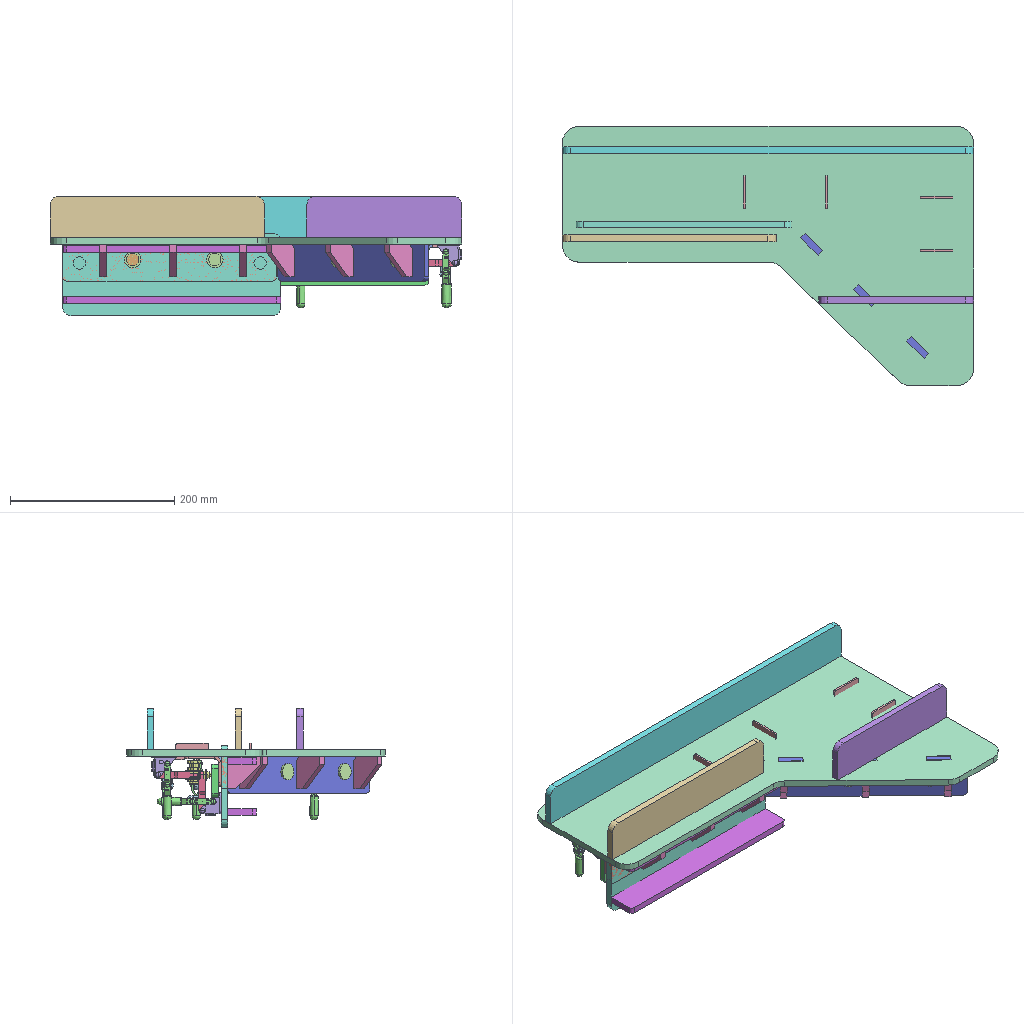Assembly | SolidWorks | 18 different items | 41 placed | box 500 x 315 x 145 mm
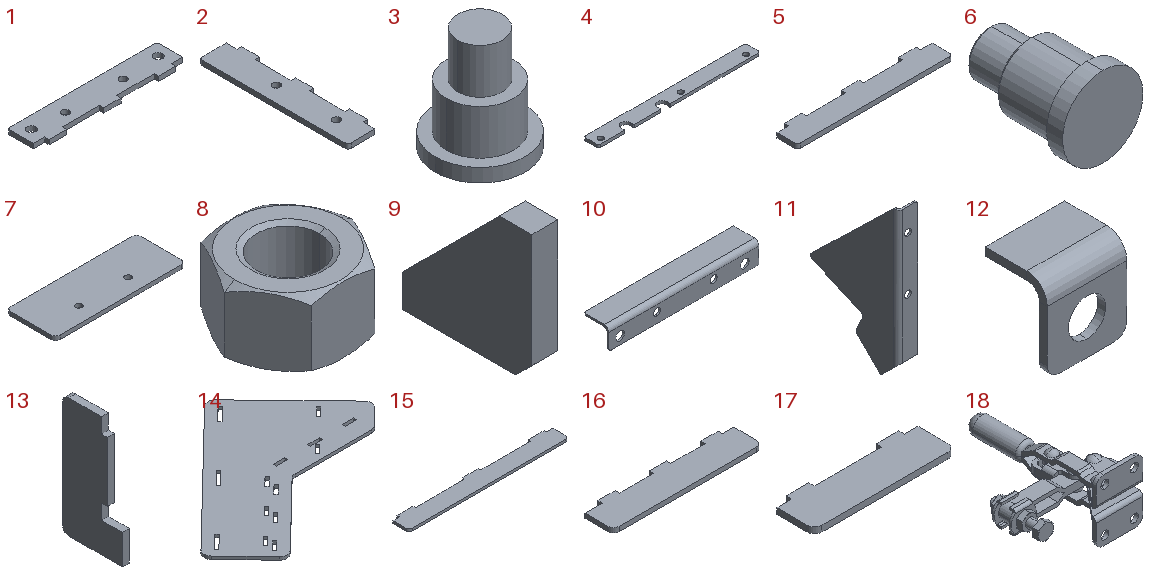Parts list (item | quantity | size | volume | features):
1 | x1 | 260 x 52.5 x 8 mm | 94123 mm3 | features FlatPattern 1, SMBaseFlange 1, SheetMetal 1
2 | x1 | 52.5 x 248 x 8 mm | 92631 mm3 | features FlatPattern 1, SMBaseFlange 1, SheetMetal 1
3 | x4 | 20 x 20 x 23 mm | 3495 mm3 | features Revolution 1
4 | x1 | 445.22 x 40 x 8 mm | 129798 mm3 | features Fillet 1, FlatPattern 1, SMBaseFlange 1, SheetMetal 1
5 | x2 | 265 x 42.5 x 8 mm | 79514 mm3 | features FlatPattern 1, SMBaseFlange 1, SheetMetal 1
6 | x3 | 15 x 21.2 x 15 mm | 2261 mm3 | features Chamfer 1, Revolution 1
7 | x1 | 265 x 100 x 8 mm | 209194 mm3 | features FlatPattern 1, ICE 1, SMBaseFlange 1, SheetMetal 1
8 | x4 | 27.713 x 24 x 14.8 mm | 5071 mm3 | features RevCut 2, Chamfer 1, Extrusion 1, LPattern 1
9 | x6 | 8 x 40 x 40 mm | 9100 mm3 | features FlatPattern 1, SMBaseFlange 1, SheetMetal 1
10 | x1 | 265 x 45 x 37 mm | 62470 mm3 | features Fillet 1, FlatPattern 1, ICE 1, SMBaseFlange 1, SheetMetal 1
11 | x1 | 37 x 163.164 x 282.329 mm | 98430 mm3 | features ICE 2, Fillet 1, FlatPattern 1, SMBaseFlange 1, SheetMetal 1
12 | x1 | 32 x 25 x 34 mm | 4824 mm3 | features Fillet 1, FlatPattern 1, ICE 1, SMBaseFlange 1, SheetMetal 1
13 | x4 | 2.3 x 20 x 40 mm | 1445 mm3 | features FlatPattern 1, SMBaseFlange 1, SheetMetal 1
14 | x1 | 561.534 x 450.241 x 8 mm | 822286 mm3 | features FlatPattern 1, SMBaseFlange 1, SheetMetal 1
15 | x1 | 500 x 57.5 x 8 mm | 208657 mm3 | features FlatPattern 1, SMBaseFlange 1, SheetMetal 1
16 | x1 | 260 x 57.5 x 8 mm | 109057 mm3 | features FlatPattern 1, SMBaseFlange 1, SheetMetal 1
17 | x1 | 188 x 57.5 x 8 mm | 78457 mm3 | features FlatPattern 1, SMBaseFlange 1, SheetMetal 1
18 | x7 | 56.45 x 77.62 x 33.3 mm | 10418 mm3 | features BaseBody 5
Mates (type | each side: item.copy, entity, surface, feature):
Coincident | 10.1 face plane Base-Flange1 | 11.1 face plane Base-Flange1
Coincident | 10.1 face plane Base-Flange1 | 11.1 face plane Cut-Extrude1 | 2 times
Coincident | 11.1 face plane Base-Flange1 | 12.1 face plane Base-Flange1
Coincident | 10.1 face plane Base-Flange1 | 12.1 face plane Base-Flange1
DistanceDim | 10.1 face plane Base-Flange1 | 12.1 face cylinder Cut-Extrude1
Concentric | 10.1 face cylinder Cut-Extrude1 | 8.1 face cone EndChamfer
Coincident | 10.1 face plane Base-Flange1 | 8.1 face plane BaseNut
Parallel | 10.1 face plane Base-Flange1 | 8.1 face plane BaseNut
Concentric | 10.1 face cylinder Cut-Extrude1 | 8.2 face cone EndChamfer
Coincident | 10.1 face plane Base-Flange1 | 8.2 face plane BaseNut
Parallel | 10.1 face plane Base-Flange1 | 8.2 face plane BaseNut
Concentric | 11.1 face cylinder Cut-Extrude2 | 8.3 face cone EndChamfer
Coincident | 11.1 face plane Base-Flange1 | 8.3 face plane BaseNut
Parallel | 11.1 face plane Base-Flange1 | 8.3 face plane BaseNut
Concentric | 11.1 face cylinder Cut-Extrude2 | 8.4 face cone EndChamfer
Coincident | 11.1 face plane Base-Flange1 | 8.4 face plane BaseNut
Parallel | 11.1 face plane Base-Flange1 | 8.4 face plane BaseNut
InPlace | 10.1 face plane Base-Flange1 | 7.1 plane
InPlace | 6.1 plane | assembly plane
Coincident | 7.1 face plane Base-Flange1 | 18.1 face plane TC1-1 vertical flange quick clamp [TCS1-1].step-1/_TCS1-1(seat).step-1-solid1
Coincident | 8.2 face plane BaseNut | 18.1 face plane TC1-1 vertical flange quick clamp [TCS1-1].step-1/_TCS1-1(bolt).step-1-solid1
DistanceDim | 18.1 face plane TC1-1 vertical flange quick clamp [TCS1-1].step-1/_TCS1-1(seat).step-1-solid1 | 7.1 face plane Base-Flange1
InPlace | 5.1 plane | assembly plane
InPlace | 11.1 face plane Base-Flange1 | 14.1 plane
InPlace | 10.1 face plane Base-Flange1 | 1.1 plane
InPlace | 11.1 face plane Base-Flange1 | 2.1 plane
Coincident | 1.1 face plane Base-Flange1 | 3.1 face plane Revolve1
Concentric | 1.1 face cylinder Base-Flange1 | 3.1 face cylinder Revolve1
Concentric | 1.1 face cylinder Base-Flange1 | 3.2 face cylinder Revolve1
Coincident | 1.1 face plane Base-Flange1 | 3.2 face plane Revolve1
Coincident | 2.1 face plane Base-Flange1 | 3.3 face plane Revolve1
Concentric | 2.1 face cylinder Base-Flange1 | 3.3 face cylinder Revolve1
Coincident | 2.1 face plane Base-Flange1 | 3.4 face plane Revolve1
Concentric | 2.1 face cylinder Base-Flange1 | 3.4 face cylinder Revolve1
Coincident | 14.1 face plane Base-Flange1 | 18.2 face plane TC1-1 vertical flange quick clamp [TCS1-1].step-1/_TCS1-1(seat).step-1-solid1
Coincident | 14.1 face plane Base-Flange1 | 18.3 face plane TC1-1 vertical flange quick clamp [TCS1-1].step-1/_TCS1-1(seat).step-1-solid1
Coincident | 14.1 face plane Base-Flange1 | 18.4 face plane TC1-1 vertical flange quick clamp [TCS1-1].step-1/_TCS1-1(seat).step-1-solid1
Coincident | 14.1 face plane Base-Flange1 | 18.5 face plane TC1-1 vertical flange quick clamp [TCS1-1].step-1/_TCS1-1(seat).step-1-solid1
Coincident | 14.1 face plane Base-Flange1 | 18.6 face plane TC1-1 vertical flange quick clamp [TCS1-1].step-1/_TCS1-1(seat).step-1-solid1
Coincident | 14.1 face plane Base-Flange1 | 9.1 face plane Base-Flange1
Coincident | 1.1 face plane Base-Flange1 | 9.1 face plane Base-Flange1
DistanceDim | 1.1 face plane Base-Flange1 | 9.1 face plane Base-Flange1
Coincident | 14.1 face plane Base-Flange1 | 9.2 face plane Base-Flange1
Coincident | 2.1 face plane Base-Flange1 | 9.2 face plane Base-Flange1
DistanceDim | 2.1 face plane Base-Flange1 | 9.2 face plane Base-Flange1
InPlace | 15.1 plane | assembly plane
InPlace | 16.1 plane | assembly plane
InPlace | 17.1 plane | assembly plane
InPlace | 10.1 face plane Base-Flange1 | 4.1 plane